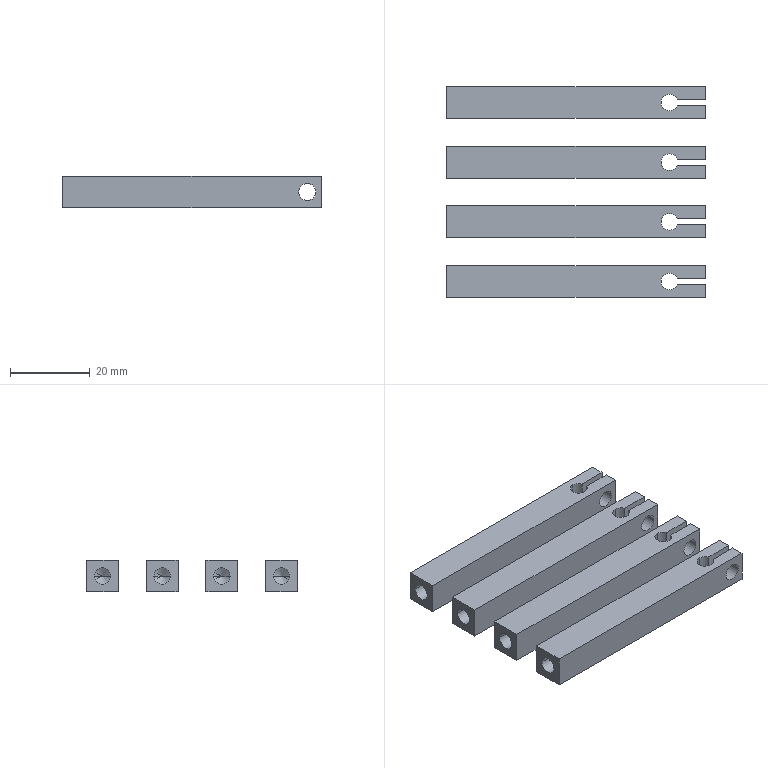Part | 4 solids | 80 faces | box 65 x 53 x 8 mm | volume 14775 mm3 | cylinder 36 | plane 36 | cone 8 | commonest cylinder face diameters 4.2 x20 4.3 x16